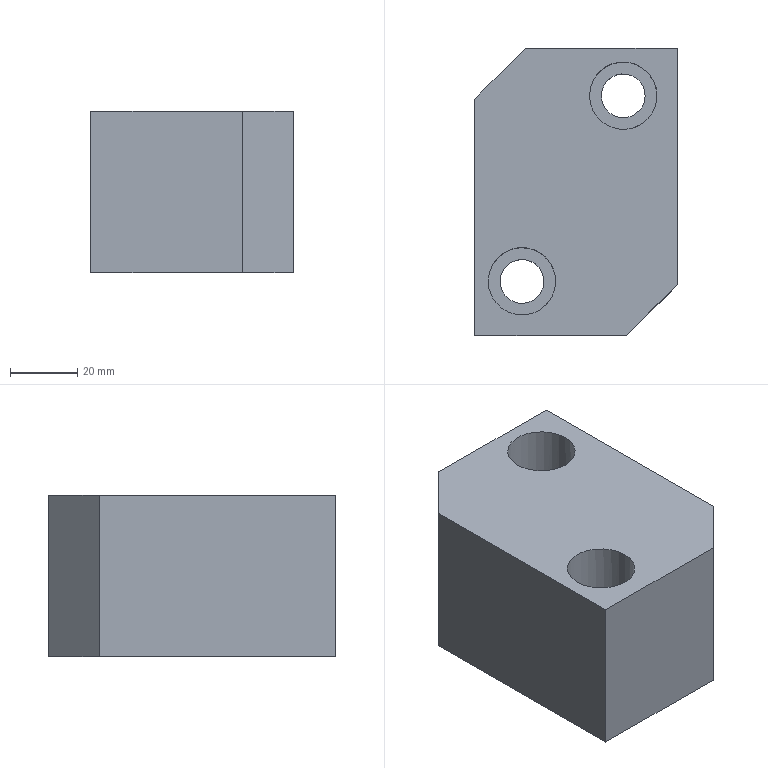Part | STEP file | gslz 2016.10.28-13_id778_x_t | 1 solid | 14 faces | box 60 x 85 x 48 mm | volume 211823 mm3 | plane 10 | cylinder 4 | commonest cylinder face diameters 13 x2 20 x2
STEP:
#1=CARTESIAN_POINT('',(0.,0.,0.));
#2=DIRECTION('',(0.,0.,1.));
#3=DIRECTION('',(1.,0.,0.));
#4=AXIS2_PLACEMENT_3D('',#1,#2,#3);
#5=CARTESIAN_POINT('',(-482.591,116.092,-48.));
#6=VERTEX_POINT('',#5);
#7=CARTESIAN_POINT('',(-481.5,122.5,-48.));
#8=DIRECTION('',(0.,0.,1.));
#9=DIRECTION('',(-0.1678,-0.9858,0.));
#10=AXIS2_PLACEMENT_3D('',#7,#8,#9);
#11=CIRCLE('',#10,6.5);
#12=CARTESIAN_POINT('',(-574.349,36.098,-48.));
#13=DIRECTION('',(0.,0.,1.));
#14=DIRECTION('',(1.,0.,0.));
#15=AXIS2_PLACEMENT_3D('',#12,#13,#14);
#16=PLANE('',#15);
#17=CARTESIAN_POINT('',(92.849,86.402));
#18=DIRECTION('',(-0.1678,-0.9858));
#19=AXIS2_PLACEMENT_2D('',#17,#18);
#20=CIRCLE('',#19,6.5);
#21=(GEOMETRIC_REPRESENTATION_CONTEXT(2)PARAMETRIC_REPRESENTATION_CONTEXT()REPRESENTATION_CONTEXT('',''));
#22=DEFINITIONAL_REPRESENTATION('',(#20),#21);
#23=PCURVE('',#16,#22);
#24=CARTESIAN_POINT('',(-481.5,122.5,-8.541));
#25=DIRECTION('',(0.,0.,-1.));
#26=DIRECTION('',(-1.,0.,0.));
#27=AXIS2_PLACEMENT_3D('',#24,#25,#26);
#28=CYLINDRICAL_SURFACE('',#27,6.5);
#29=CARTESIAN_POINT('',(11.164,39.459));
#30=DIRECTION('',(-1.,0.));
#31=VECTOR('',#30,1.);
#32=LINE('',#29,#31);
#33=(GEOMETRIC_REPRESENTATION_CONTEXT(2)PARAMETRIC_REPRESENTATION_CONTEXT()REPRESENTATION_CONTEXT('',''));
#34=DEFINITIONAL_REPRESENTATION('',(#32),#33);
#35=PCURVE('',#28,#34);
#36=SURFACE_CURVE('',#11,(#23,#35),.PCURVE_S1.);
#37=EDGE_CURVE('',#6,#6,#36,.T.);
#38=ORIENTED_EDGE('',*,*,#37,.T.);
#39=EDGE_LOOP('',(#38));
#40=FACE_BOUND('',#39,.T.);
#41=CARTESIAN_POINT('',(-452.591,171.092,-48.));
#42=VERTEX_POINT('',#41);
#43=CARTESIAN_POINT('',(-451.5,177.5,-48.));
#44=DIRECTION('',(0.,0.,1.));
#45=DIRECTION('',(-0.1678,-0.9858,0.));
#46=AXIS2_PLACEMENT_3D('',#43,#44,#45);
#47=CIRCLE('',#46,6.5);
#48=CARTESIAN_POINT('',(122.849,141.402));
#49=DIRECTION('',(-0.1678,-0.9858));
#50=AXIS2_PLACEMENT_2D('',#48,#49);
#51=CIRCLE('',#50,6.5);
#52=(GEOMETRIC_REPRESENTATION_CONTEXT(2)PARAMETRIC_REPRESENTATION_CONTEXT()REPRESENTATION_CONTEXT('',''));
#53=DEFINITIONAL_REPRESENTATION('',(#51),#52);
#54=PCURVE('',#16,#53);
#55=CARTESIAN_POINT('',(-451.5,177.5,-8.541));
#56=DIRECTION('',(0.,0.,-1.));
#57=DIRECTION('',(-1.,0.,0.));
#58=AXIS2_PLACEMENT_3D('',#55,#56,#57);
#59=CYLINDRICAL_SURFACE('',#58,6.5);
#60=CARTESIAN_POINT('',(11.164,39.459));
#61=DIRECTION('',(-1.,0.));
#62=VECTOR('',#61,1.);
#63=LINE('',#60,#62);
#64=(GEOMETRIC_REPRESENTATION_CONTEXT(2)PARAMETRIC_REPRESENTATION_CONTEXT()REPRESENTATION_CONTEXT('',''));
#65=DEFINITIONAL_REPRESENTATION('',(#63),#64);
#66=PCURVE('',#59,#65);
#67=SURFACE_CURVE('',#47,(#54,#66),.PCURVE_S1.);
#68=EDGE_CURVE('',#42,#42,#67,.T.);
#69=ORIENTED_EDGE('',*,*,#68,.T.);
#70=EDGE_LOOP('',(#69));
#71=FACE_BOUND('',#70,.T.);
#72=CARTESIAN_POINT('',(-495.5,176.5,-48.));
#73=VERTEX_POINT('',#72);
#74=CARTESIAN_POINT('',(-495.5,106.5,-48.));
#75=VERTEX_POINT('',#74);
#76=CARTESIAN_POINT('',(-495.5,151.5,-48.));
#77=DIRECTION('',(0.,-1.,0.));
#78=VECTOR('',#77,1.);
#79=LINE('',#76,#78);
#80=CARTESIAN_POINT('',(78.849,115.402));
#81=DIRECTION('',(0.,-1.));
#82=VECTOR('',#81,1.);
#83=LINE('',#80,#82);
#84=(GEOMETRIC_REPRESENTATION_CONTEXT(2)PARAMETRIC_REPRESENTATION_CONTEXT()REPRESENTATION_CONTEXT('',''));
#85=DEFINITIONAL_REPRESENTATION('',(#83),#84);
#86=PCURVE('',#16,#85);
#87=CARTESIAN_POINT('',(-495.5,151.5,-25.5));
#88=DIRECTION('',(1.,0.,0.));
#89=DIRECTION('',(0.,0.,-1.));
#90=AXIS2_PLACEMENT_3D('',#87,#88,#89);
#91=PLANE('',#90);
#92=CARTESIAN_POINT('',(22.5,0.));
#93=DIRECTION('',(0.,-1.));
#94=VECTOR('',#93,1.);
#95=LINE('',#92,#94);
#96=(GEOMETRIC_REPRESENTATION_CONTEXT(2)PARAMETRIC_REPRESENTATION_CONTEXT()REPRESENTATION_CONTEXT('',''));
#97=DEFINITIONAL_REPRESENTATION('',(#95),#96);
#98=PCURVE('',#91,#97);
#99=SURFACE_CURVE('',#79,(#86,#98),.PCURVE_S1.);
#100=EDGE_CURVE('',#73,#75,#99,.T.);
#101=ORIENTED_EDGE('',*,*,#100,.F.);
#102=CARTESIAN_POINT('',(-480.5,191.5,-48.));
#103=VERTEX_POINT('',#102);
#104=CARTESIAN_POINT('',(-495.5,176.5,-48.));
#105=DIRECTION('',(0.7071,0.7071,0.));
#106=VECTOR('',#105,1.);
#107=LINE('',#104,#106);
#108=CARTESIAN_POINT('',(78.849,140.402));
#109=DIRECTION('',(0.7071,0.7071));
#110=VECTOR('',#109,1.);
#111=LINE('',#108,#110);
#112=(GEOMETRIC_REPRESENTATION_CONTEXT(2)PARAMETRIC_REPRESENTATION_CONTEXT()REPRESENTATION_CONTEXT('',''));
#113=DEFINITIONAL_REPRESENTATION('',(#111),#112);
#114=PCURVE('',#16,#113);
#115=CARTESIAN_POINT('',(-495.5,176.5,-25.5));
#116=DIRECTION('',(-0.7071,0.7071,0.));
#117=DIRECTION('',(0.,0.,1.));
#118=AXIS2_PLACEMENT_3D('',#115,#116,#117);
#119=PLANE('',#118);
#120=CARTESIAN_POINT('',(-22.5,0.));
#121=DIRECTION('',(0.,1.));
#122=VECTOR('',#121,1.);
#123=LINE('',#120,#122);
#124=(GEOMETRIC_REPRESENTATION_CONTEXT(2)PARAMETRIC_REPRESENTATION_CONTEXT()REPRESENTATION_CONTEXT('',''));
#125=DEFINITIONAL_REPRESENTATION('',(#123),#124);
#126=PCURVE('',#119,#125);
#127=SURFACE_CURVE('',#107,(#114,#126),.PCURVE_S1.);
#128=EDGE_CURVE('',#73,#103,#127,.T.);
#129=ORIENTED_EDGE('',*,*,#128,.T.);
#130=CARTESIAN_POINT('',(-435.5,191.5,-48.));
#131=VERTEX_POINT('',#130);
#132=CARTESIAN_POINT('',(-574.349,191.5,-48.));
#133=DIRECTION('',(-1.,0.,0.));
#134=VECTOR('',#133,1.);
#135=LINE('',#132,#134);
#136=CARTESIAN_POINT('',(0.,155.402));
#137=DIRECTION('',(-1.,0.));
#138=VECTOR('',#137,1.);
#139=LINE('',#136,#138);
#140=(GEOMETRIC_REPRESENTATION_CONTEXT(2)PARAMETRIC_REPRESENTATION_CONTEXT()REPRESENTATION_CONTEXT('',''));
#141=DEFINITIONAL_REPRESENTATION('',(#139),#140);
#142=PCURVE('',#16,#141);
#143=CARTESIAN_POINT('',(-441.5,191.5,-43.));
#144=DIRECTION('',(0.,1.,0.));
#145=DIRECTION('',(-1.,0.,0.));
#146=AXIS2_PLACEMENT_3D('',#143,#144,#145);
#147=PLANE('',#146);
#148=CARTESIAN_POINT('',(132.849,-5.));
#149=DIRECTION('',(1.,0.));
#150=VECTOR('',#149,1.);
#151=LINE('',#148,#150);
#152=(GEOMETRIC_REPRESENTATION_CONTEXT(2)PARAMETRIC_REPRESENTATION_CONTEXT()REPRESENTATION_CONTEXT('',''));
#153=DEFINITIONAL_REPRESENTATION('',(#151),#152);
#154=PCURVE('',#147,#153);
#155=SURFACE_CURVE('',#135,(#142,#154),.PCURVE_S1.);
#156=EDGE_CURVE('',#131,#103,#155,.T.);
#157=ORIENTED_EDGE('',*,*,#156,.F.);
#158=CARTESIAN_POINT('',(-435.5,121.5,-48.));
#159=VERTEX_POINT('',#158);
#160=CARTESIAN_POINT('',(-435.5,36.098,-48.));
#161=DIRECTION('',(0.,1.,0.));
#162=VECTOR('',#161,1.);
#163=LINE('',#160,#162);
#164=CARTESIAN_POINT('',(138.849,0.));
#165=DIRECTION('',(0.,1.));
#166=VECTOR('',#165,1.);
#167=LINE('',#164,#166);
#168=(GEOMETRIC_REPRESENTATION_CONTEXT(2)PARAMETRIC_REPRESENTATION_CONTEXT()REPRESENTATION_CONTEXT('',''));
#169=DEFINITIONAL_REPRESENTATION('',(#167),#168);
#170=PCURVE('',#16,#169);
#171=CARTESIAN_POINT('',(-435.5,106.5,-43.));
#172=DIRECTION('',(1.,0.,0.));
#173=DIRECTION('',(0.,1.,0.));
#174=AXIS2_PLACEMENT_3D('',#171,#172,#173);
#175=PLANE('',#174);
#176=CARTESIAN_POINT('',(-70.402,-5.));
#177=DIRECTION('',(1.,0.));
#178=VECTOR('',#177,1.);
#179=LINE('',#176,#178);
#180=(GEOMETRIC_REPRESENTATION_CONTEXT(2)PARAMETRIC_REPRESENTATION_CONTEXT()REPRESENTATION_CONTEXT('',''));
#181=DEFINITIONAL_REPRESENTATION('',(#179),#180);
#182=PCURVE('',#175,#181);
#183=SURFACE_CURVE('',#163,(#170,#182),.PCURVE_S1.);
#184=EDGE_CURVE('',#159,#131,#183,.T.);
#185=ORIENTED_EDGE('',*,*,#184,.F.);
#186=CARTESIAN_POINT('',(-450.5,106.5,-48.));
#187=VERTEX_POINT('',#186);
#188=CARTESIAN_POINT('',(-450.5,106.5,-48.));
#189=DIRECTION('',(-0.7071,-0.7071,0.));
#190=VECTOR('',#189,1.);
#191=LINE('',#188,#190);
#192=CARTESIAN_POINT('',(123.849,70.402));
#193=DIRECTION('',(-0.7071,-0.7071));
#194=VECTOR('',#193,1.);
#195=LINE('',#192,#194);
#196=(GEOMETRIC_REPRESENTATION_CONTEXT(2)PARAMETRIC_REPRESENTATION_CONTEXT()REPRESENTATION_CONTEXT('',''));
#197=DEFINITIONAL_REPRESENTATION('',(#195),#196);
#198=PCURVE('',#16,#197);
#199=CARTESIAN_POINT('',(-450.5,106.5,-43.));
#200=DIRECTION('',(-0.7071,0.7071,0.));
#201=DIRECTION('',(0.,0.,1.));
#202=AXIS2_PLACEMENT_3D('',#199,#200,#201);
#203=PLANE('',#202);
#204=CARTESIAN_POINT('',(-5.,0.));
#205=DIRECTION('',(0.,-1.));
#206=VECTOR('',#205,1.);
#207=LINE('',#204,#206);
#208=(GEOMETRIC_REPRESENTATION_CONTEXT(2)PARAMETRIC_REPRESENTATION_CONTEXT()REPRESENTATION_CONTEXT('',''));
#209=DEFINITIONAL_REPRESENTATION('',(#207),#208);
#210=PCURVE('',#203,#209);
#211=SURFACE_CURVE('',#191,(#198,#210),.PCURVE_S1.);
#212=EDGE_CURVE('',#159,#187,#211,.T.);
#213=ORIENTED_EDGE('',*,*,#212,.T.);
#214=CARTESIAN_POINT('',(-574.349,106.5,-48.));
#215=DIRECTION('',(1.,0.,0.));
#216=VECTOR('',#215,1.);
#217=LINE('',#214,#216);
#218=CARTESIAN_POINT('',(0.,70.402));
#219=DIRECTION('',(1.,0.));
#220=VECTOR('',#219,1.);
#221=LINE('',#218,#220);
#222=(GEOMETRIC_REPRESENTATION_CONTEXT(2)PARAMETRIC_REPRESENTATION_CONTEXT()REPRESENTATION_CONTEXT('',''));
#223=DEFINITIONAL_REPRESENTATION('',(#221),#222);
#224=PCURVE('',#16,#223);
#225=CARTESIAN_POINT('',(-631.5,106.5,-43.));
#226=DIRECTION('',(0.,-1.,0.));
#227=DIRECTION('',(0.,0.,1.));
#228=AXIS2_PLACEMENT_3D('',#225,#226,#227);
#229=PLANE('',#228);
#230=CARTESIAN_POINT('',(-5.,-57.151));
#231=DIRECTION('',(0.,-1.));
#232=VECTOR('',#231,1.);
#233=LINE('',#230,#232);
#234=(GEOMETRIC_REPRESENTATION_CONTEXT(2)PARAMETRIC_REPRESENTATION_CONTEXT()REPRESENTATION_CONTEXT('',''));
#235=DEFINITIONAL_REPRESENTATION('',(#233),#234);
#236=PCURVE('',#229,#235);
#237=SURFACE_CURVE('',#217,(#224,#236),.PCURVE_S1.);
#238=EDGE_CURVE('',#75,#187,#237,.T.);
#239=ORIENTED_EDGE('',*,*,#238,.F.);
#240=EDGE_LOOP('',(#101,#129,#157,#185,#213,#239));
#241=FACE_BOUND('',#240,.T.);
#242=ADVANCED_FACE('',(#40,#71,#241),#16,.F.);
#243=ORIENTED_EDGE('',*,*,#156,.T.);
#244=CARTESIAN_POINT('',(-480.5,191.5,0.));
#245=VERTEX_POINT('',#244);
#246=CARTESIAN_POINT('',(-480.5,191.5,0.));
#247=DIRECTION('',(0.,0.,1.));
#248=VECTOR('',#247,1.);
#249=LINE('',#246,#248);
#250=CARTESIAN_POINT('',(39.,43.));
#251=DIRECTION('',(0.,1.));
#252=VECTOR('',#251,1.);
#253=LINE('',#250,#252);
#254=(GEOMETRIC_REPRESENTATION_CONTEXT(2)PARAMETRIC_REPRESENTATION_CONTEXT()REPRESENTATION_CONTEXT('',''));
#255=DEFINITIONAL_REPRESENTATION('',(#253),#254);
#256=PCURVE('',#147,#255);
#257=CARTESIAN_POINT('',(25.5,21.213));
#258=DIRECTION('',(1.,0.));
#259=VECTOR('',#258,1.);
#260=LINE('',#257,#259);
#261=(GEOMETRIC_REPRESENTATION_CONTEXT(2)PARAMETRIC_REPRESENTATION_CONTEXT()REPRESENTATION_CONTEXT('',''));
#262=DEFINITIONAL_REPRESENTATION('',(#260),#261);
#263=PCURVE('',#119,#262);
#264=SURFACE_CURVE('',#249,(#256,#263),.PCURVE_S1.);
#265=EDGE_CURVE('',#103,#245,#264,.T.);
#266=ORIENTED_EDGE('',*,*,#265,.T.);
#267=CARTESIAN_POINT('',(-435.5,191.5,0.));
#268=VERTEX_POINT('',#267);
#269=CARTESIAN_POINT('',(-441.5,191.5,0.));
#270=DIRECTION('',(-1.,0.,0.));
#271=VECTOR('',#270,1.);
#272=LINE('',#269,#271);
#273=CARTESIAN_POINT('',(0.,43.));
#274=DIRECTION('',(1.,0.));
#275=VECTOR('',#274,1.);
#276=LINE('',#273,#275);
#277=(GEOMETRIC_REPRESENTATION_CONTEXT(2)PARAMETRIC_REPRESENTATION_CONTEXT()REPRESENTATION_CONTEXT('',''));
#278=DEFINITIONAL_REPRESENTATION('',(#276),#277);
#279=PCURVE('',#147,#278);
#280=CARTESIAN_POINT('',(-540.228,222.5,0.));
#281=DIRECTION('',(0.,0.,1.));
#282=DIRECTION('',(0.,1.,0.));
#283=AXIS2_PLACEMENT_3D('',#280,#281,#282);
#284=PLANE('',#283);
#285=CARTESIAN_POINT('',(-31.,-98.728));
#286=DIRECTION('',(0.,1.));
#287=VECTOR('',#286,1.);
#288=LINE('',#285,#287);
#289=(GEOMETRIC_REPRESENTATION_CONTEXT(2)PARAMETRIC_REPRESENTATION_CONTEXT()REPRESENTATION_CONTEXT('',''));
#290=DEFINITIONAL_REPRESENTATION('',(#288),#289);
#291=PCURVE('',#284,#290);
#292=SURFACE_CURVE('',#272,(#279,#291),.PCURVE_S1.);
#293=EDGE_CURVE('',#268,#245,#292,.T.);
#294=ORIENTED_EDGE('',*,*,#293,.F.);
#295=CARTESIAN_POINT('',(-435.5,191.5,-43.));
#296=DIRECTION('',(0.,0.,1.));
#297=VECTOR('',#296,1.);
#298=LINE('',#295,#297);
#299=CARTESIAN_POINT('',(-6.,0.));
#300=DIRECTION('',(0.,1.));
#301=VECTOR('',#300,1.);
#302=LINE('',#299,#301);
#303=(GEOMETRIC_REPRESENTATION_CONTEXT(2)PARAMETRIC_REPRESENTATION_CONTEXT()REPRESENTATION_CONTEXT('',''));
#304=DEFINITIONAL_REPRESENTATION('',(#302),#303);
#305=PCURVE('',#147,#304);
#306=CARTESIAN_POINT('',(85.,0.));
#307=DIRECTION('',(0.,1.));
#308=VECTOR('',#307,1.);
#309=LINE('',#306,#308);
#310=(GEOMETRIC_REPRESENTATION_CONTEXT(2)PARAMETRIC_REPRESENTATION_CONTEXT()REPRESENTATION_CONTEXT('',''));
#311=DEFINITIONAL_REPRESENTATION('',(#309),#310);
#312=PCURVE('',#175,#311);
#313=SURFACE_CURVE('',#298,(#305,#312),.PCURVE_S1.);
#314=EDGE_CURVE('',#131,#268,#313,.T.);
#315=ORIENTED_EDGE('',*,*,#314,.F.);
#316=EDGE_LOOP('',(#243,#266,#294,#315));
#317=FACE_BOUND('',#316,.T.);
#318=ADVANCED_FACE('',(#317),#147,.T.);
#319=CARTESIAN_POINT('',(-435.5,121.5,0.));
#320=VERTEX_POINT('',#319);
#321=CARTESIAN_POINT('',(-435.5,106.5,0.));
#322=DIRECTION('',(0.,1.,0.));
#323=VECTOR('',#322,1.);
#324=LINE('',#321,#323);
#325=CARTESIAN_POINT('',(0.,43.));
#326=DIRECTION('',(1.,0.));
#327=VECTOR('',#326,1.);
#328=LINE('',#325,#327);
#329=(GEOMETRIC_REPRESENTATION_CONTEXT(2)PARAMETRIC_REPRESENTATION_CONTEXT()REPRESENTATION_CONTEXT('',''));
#330=DEFINITIONAL_REPRESENTATION('',(#328),#329);
#331=PCURVE('',#175,#330);
#332=CARTESIAN_POINT('',(-116.,-104.728));
#333=DIRECTION('',(1.,0.));
#334=VECTOR('',#333,1.);
#335=LINE('',#332,#334);
#336=(GEOMETRIC_REPRESENTATION_CONTEXT(2)PARAMETRIC_REPRESENTATION_CONTEXT()REPRESENTATION_CONTEXT('',''));
#337=DEFINITIONAL_REPRESENTATION('',(#335),#336);
#338=PCURVE('',#284,#337);
#339=SURFACE_CURVE('',#324,(#331,#338),.PCURVE_S1.);
#340=EDGE_CURVE('',#320,#268,#339,.T.);
#341=ORIENTED_EDGE('',*,*,#340,.F.);
#342=CARTESIAN_POINT('',(-435.5,121.5,-43.));
#343=DIRECTION('',(0.,0.,-1.));
#344=VECTOR('',#343,1.);
#345=LINE('',#342,#344);
#346=CARTESIAN_POINT('',(15.,0.));
#347=DIRECTION('',(0.,-1.));
#348=VECTOR('',#347,1.);
#349=LINE('',#346,#348);
#350=(GEOMETRIC_REPRESENTATION_CONTEXT(2)PARAMETRIC_REPRESENTATION_CONTEXT()REPRESENTATION_CONTEXT('',''));
#351=DEFINITIONAL_REPRESENTATION('',(#349),#350);
#352=PCURVE('',#175,#351);
#353=CARTESIAN_POINT('',(0.,21.213));
#354=DIRECTION('',(-1.,0.));
#355=VECTOR('',#354,1.);
#356=LINE('',#353,#355);
#357=(GEOMETRIC_REPRESENTATION_CONTEXT(2)PARAMETRIC_REPRESENTATION_CONTEXT()REPRESENTATION_CONTEXT('',''));
#358=DEFINITIONAL_REPRESENTATION('',(#356),#357);
#359=PCURVE('',#203,#358);
#360=SURFACE_CURVE('',#345,(#352,#359),.PCURVE_S1.);
#361=EDGE_CURVE('',#320,#159,#360,.T.);
#362=ORIENTED_EDGE('',*,*,#361,.T.);
#363=ORIENTED_EDGE('',*,*,#184,.T.);
#364=ORIENTED_EDGE('',*,*,#314,.T.);
#365=EDGE_LOOP('',(#341,#362,#363,#364));
#366=FACE_BOUND('',#365,.T.);
#367=ADVANCED_FACE('',(#366),#175,.T.);
#368=ORIENTED_EDGE('',*,*,#238,.T.);
#369=CARTESIAN_POINT('',(-450.5,106.5,0.));
#370=VERTEX_POINT('',#369);
#371=CARTESIAN_POINT('',(-450.5,106.5,-43.));
#372=DIRECTION('',(0.,0.,1.));
#373=VECTOR('',#372,1.);
#374=LINE('',#371,#373);
#375=CARTESIAN_POINT('',(0.,-181.));
#376=DIRECTION('',(1.,0.));
#377=VECTOR('',#376,1.);
#378=LINE('',#375,#377);
#379=(GEOMETRIC_REPRESENTATION_CONTEXT(2)PARAMETRIC_REPRESENTATION_CONTEXT()REPRESENTATION_CONTEXT('',''));
#380=DEFINITIONAL_REPRESENTATION('',(#378),#379);
#381=PCURVE('',#229,#380);
#382=CARTESIAN_POINT('',(0.,0.));
#383=DIRECTION('',(1.,0.));
#384=VECTOR('',#383,1.);
#385=LINE('',#382,#384);
#386=(GEOMETRIC_REPRESENTATION_CONTEXT(2)PARAMETRIC_REPRESENTATION_CONTEXT()REPRESENTATION_CONTEXT('',''));
#387=DEFINITIONAL_REPRESENTATION('',(#385),#386);
#388=PCURVE('',#203,#387);
#389=SURFACE_CURVE('',#374,(#381,#388),.PCURVE_S1.);
#390=EDGE_CURVE('',#187,#370,#389,.T.);
#391=ORIENTED_EDGE('',*,*,#390,.T.);
#392=CARTESIAN_POINT('',(-495.5,106.5,0.));
#393=VERTEX_POINT('',#392);
#394=CARTESIAN_POINT('',(-631.5,106.5,0.));
#395=DIRECTION('',(1.,0.,0.));
#396=VECTOR('',#395,1.);
#397=LINE('',#394,#396);
#398=CARTESIAN_POINT('',(43.,0.));
#399=DIRECTION('',(0.,-1.));
#400=VECTOR('',#399,1.);
#401=LINE('',#398,#400);
#402=(GEOMETRIC_REPRESENTATION_CONTEXT(2)PARAMETRIC_REPRESENTATION_CONTEXT()REPRESENTATION_CONTEXT('',''));
#403=DEFINITIONAL_REPRESENTATION('',(#401),#402);
#404=PCURVE('',#229,#403);
#405=CARTESIAN_POINT('',(-116.,91.272));
#406=DIRECTION('',(0.,-1.));
#407=VECTOR('',#406,1.);
#408=LINE('',#405,#407);
#409=(GEOMETRIC_REPRESENTATION_CONTEXT(2)PARAMETRIC_REPRESENTATION_CONTEXT()REPRESENTATION_CONTEXT('',''));
#410=DEFINITIONAL_REPRESENTATION('',(#408),#409);
#411=PCURVE('',#284,#410);
#412=SURFACE_CURVE('',#397,(#404,#411),.PCURVE_S1.);
#413=EDGE_CURVE('',#393,#370,#412,.T.);
#414=ORIENTED_EDGE('',*,*,#413,.F.);
#415=CARTESIAN_POINT('',(-495.5,106.5,-43.));
#416=DIRECTION('',(0.,0.,-1.));
#417=VECTOR('',#416,1.);
#418=LINE('',#415,#417);
#419=CARTESIAN_POINT('',(0.,-136.));
#420=DIRECTION('',(-1.,0.));
#421=VECTOR('',#420,1.);
#422=LINE('',#419,#421);
#423=(GEOMETRIC_REPRESENTATION_CONTEXT(2)PARAMETRIC_REPRESENTATION_CONTEXT()REPRESENTATION_CONTEXT('',''));
#424=DEFINITIONAL_REPRESENTATION('',(#422),#423);
#425=PCURVE('',#229,#424);
#426=CARTESIAN_POINT('',(17.5,-45.));
#427=DIRECTION('',(1.,0.));
#428=VECTOR('',#427,1.);
#429=LINE('',#426,#428);
#430=(GEOMETRIC_REPRESENTATION_CONTEXT(2)PARAMETRIC_REPRESENTATION_CONTEXT()REPRESENTATION_CONTEXT('',''));
#431=DEFINITIONAL_REPRESENTATION('',(#429),#430);
#432=PCURVE('',#91,#431);
#433=SURFACE_CURVE('',#418,(#425,#432),.PCURVE_S1.);
#434=EDGE_CURVE('',#393,#75,#433,.T.);
#435=ORIENTED_EDGE('',*,*,#434,.T.);
#436=EDGE_LOOP('',(#368,#391,#414,#435));
#437=FACE_BOUND('',#436,.T.);
#438=ADVANCED_FACE('',(#437),#229,.T.);
#439=CARTESIAN_POINT('',(-495.5,176.5,0.));
#440=VERTEX_POINT('',#439);
#441=CARTESIAN_POINT('',(-495.5,222.5,0.));
#442=DIRECTION('',(0.,1.,0.));
#443=VECTOR('',#442,1.);
#444=LINE('',#441,#443);
#445=CARTESIAN_POINT('',(-25.5,71.));
#446=DIRECTION('',(0.,1.));
#447=VECTOR('',#446,1.);
#448=LINE('',#445,#447);
#449=(GEOMETRIC_REPRESENTATION_CONTEXT(2)PARAMETRIC_REPRESENTATION_CONTEXT()REPRESENTATION_CONTEXT('',''));
#450=DEFINITIONAL_REPRESENTATION('',(#448),#449);
#451=PCURVE('',#91,#450);
#452=CARTESIAN_POINT('',(0.,-44.728));
#453=DIRECTION('',(1.,0.));
#454=VECTOR('',#453,1.);
#455=LINE('',#452,#454);
#456=(GEOMETRIC_REPRESENTATION_CONTEXT(2)PARAMETRIC_REPRESENTATION_CONTEXT()REPRESENTATION_CONTEXT('',''));
#457=DEFINITIONAL_REPRESENTATION('',(#455),#456);
#458=PCURVE('',#284,#457);
#459=SURFACE_CURVE('',#444,(#451,#458),.PCURVE_S1.);
#460=EDGE_CURVE('',#393,#440,#459,.T.);
#461=ORIENTED_EDGE('',*,*,#460,.T.);
#462=CARTESIAN_POINT('',(-495.5,176.5,-48.));
#463=DIRECTION('',(0.,0.,-1.));
#464=VECTOR('',#463,1.);
#465=LINE('',#462,#464);
#466=CARTESIAN_POINT('',(22.5,25.));
#467=DIRECTION('',(1.,0.));
#468=VECTOR('',#467,1.);
#469=LINE('',#466,#468);
#470=(GEOMETRIC_REPRESENTATION_CONTEXT(2)PARAMETRIC_REPRESENTATION_CONTEXT()REPRESENTATION_CONTEXT('',''));
#471=DEFINITIONAL_REPRESENTATION('',(#469),#470);
#472=PCURVE('',#91,#471);
#473=CARTESIAN_POINT('',(-22.5,0.));
#474=DIRECTION('',(-1.,0.));
#475=VECTOR('',#474,1.);
#476=LINE('',#473,#475);
#477=(GEOMETRIC_REPRESENTATION_CONTEXT(2)PARAMETRIC_REPRESENTATION_CONTEXT()REPRESENTATION_CONTEXT('',''));
#478=DEFINITIONAL_REPRESENTATION('',(#476),#477);
#479=PCURVE('',#119,#478);
#480=SURFACE_CURVE('',#465,(#472,#479),.PCURVE_S1.);
#481=EDGE_CURVE('',#440,#73,#480,.T.);
#482=ORIENTED_EDGE('',*,*,#481,.T.);
#483=ORIENTED_EDGE('',*,*,#100,.T.);
#484=ORIENTED_EDGE('',*,*,#434,.F.);
#485=EDGE_LOOP('',(#461,#482,#483,#484));
#486=FACE_BOUND('',#485,.T.);
#487=ADVANCED_FACE('',(#486),#91,.F.);
#488=CARTESIAN_POINT('',(-471.5,122.5,0.));
#489=VERTEX_POINT('',#488);
#490=CARTESIAN_POINT('',(-483.178,112.642,0.));
#491=VERTEX_POINT('',#490);
#492=CARTESIAN_POINT('',(-481.5,122.5,0.));
#493=DIRECTION('',(0.,0.,1.));
#494=DIRECTION('',(1.,0.,0.));
#495=AXIS2_PLACEMENT_3D('',#492,#493,#494);
#496=CIRCLE('',#495,10.);
#497=CARTESIAN_POINT('',(-100.,-58.728));
#498=DIRECTION('',(0.,-1.));
#499=AXIS2_PLACEMENT_2D('',#497,#498);
#500=CIRCLE('',#499,10.);
#501=(GEOMETRIC_REPRESENTATION_CONTEXT(2)PARAMETRIC_REPRESENTATION_CONTEXT()REPRESENTATION_CONTEXT('',''));
#502=DEFINITIONAL_REPRESENTATION('',(#500),#501);
#503=PCURVE('',#284,#502);
#504=CARTESIAN_POINT('',(-481.5,122.5,-8.541));
#505=DIRECTION('',(0.,0.,-1.));
#506=DIRECTION('',(-1.,0.,0.));
#507=AXIS2_PLACEMENT_3D('',#504,#505,#506);
#508=CYLINDRICAL_SURFACE('',#507,10.);
#509=CARTESIAN_POINT('',(9.425,-8.541));
#510=DIRECTION('',(-1.,0.));
#511=VECTOR('',#510,1.);
#512=LINE('',#509,#511);
#513=(GEOMETRIC_REPRESENTATION_CONTEXT(2)PARAMETRIC_REPRESENTATION_CONTEXT()REPRESENTATION_CONTEXT('',''));
#514=DEFINITIONAL_REPRESENTATION('',(#512),#513);
#515=PCURVE('',#508,#514);
#516=SURFACE_CURVE('',#496,(#503,#515),.PCURVE_S1.);
#517=EDGE_CURVE('',#489,#491,#516,.T.);
#518=ORIENTED_EDGE('',*,*,#517,.F.);
#519=CARTESIAN_POINT('',(-481.5,122.5,0.));
#520=DIRECTION('',(0.,0.,1.));
#521=DIRECTION('',(1.,0.,0.));
#522=AXIS2_PLACEMENT_3D('',#519,#520,#521);
#523=CIRCLE('',#522,10.);
#524=CARTESIAN_POINT('',(-100.,-58.728));
#525=DIRECTION('',(0.,-1.));
#526=AXIS2_PLACEMENT_2D('',#524,#525);
#527=CIRCLE('',#526,10.);
#528=(GEOMETRIC_REPRESENTATION_CONTEXT(2)PARAMETRIC_REPRESENTATION_CONTEXT()REPRESENTATION_CONTEXT('',''));
#529=DEFINITIONAL_REPRESENTATION('',(#527),#528);
#530=PCURVE('',#284,#529);
#531=CARTESIAN_POINT('',(15.708,-8.541));
#532=DIRECTION('',(-1.,0.));
#533=VECTOR('',#532,1.);
#534=LINE('',#531,#533);
#535=(GEOMETRIC_REPRESENTATION_CONTEXT(2)PARAMETRIC_REPRESENTATION_CONTEXT()REPRESENTATION_CONTEXT('',''));
#536=DEFINITIONAL_REPRESENTATION('',(#534),#535);
#537=PCURVE('',#508,#536);
#538=SURFACE_CURVE('',#523,(#530,#537),.PCURVE_S1.);
#539=EDGE_CURVE('',#491,#489,#538,.T.);
#540=ORIENTED_EDGE('',*,*,#539,.F.);
#541=EDGE_LOOP('',(#518,#540));
#542=FACE_BOUND('',#541,.T.);
#543=CARTESIAN_POINT('',(-441.5,177.5,0.));
#544=VERTEX_POINT('',#543);
#545=CARTESIAN_POINT('',(-453.178,167.642,0.));
#546=VERTEX_POINT('',#545);
#547=CARTESIAN_POINT('',(-451.5,177.5,0.));
#548=DIRECTION('',(0.,0.,1.));
#549=DIRECTION('',(1.,0.,0.));
#550=AXIS2_PLACEMENT_3D('',#547,#548,#549);
#551=CIRCLE('',#550,10.);
#552=CARTESIAN_POINT('',(-45.,-88.728));
#553=DIRECTION('',(0.,-1.));
#554=AXIS2_PLACEMENT_2D('',#552,#553);
#555=CIRCLE('',#554,10.);
#556=(GEOMETRIC_REPRESENTATION_CONTEXT(2)PARAMETRIC_REPRESENTATION_CONTEXT()REPRESENTATION_CONTEXT('',''));
#557=DEFINITIONAL_REPRESENTATION('',(#555),#556);
#558=PCURVE('',#284,#557);
#559=CARTESIAN_POINT('',(-451.5,177.5,-8.541));
#560=DIRECTION('',(0.,0.,-1.));
#561=DIRECTION('',(-1.,0.,0.));
#562=AXIS2_PLACEMENT_3D('',#559,#560,#561);
#563=CYLINDRICAL_SURFACE('',#562,10.);
#564=CARTESIAN_POINT('',(9.425,-8.541));
#565=DIRECTION('',(-1.,0.));
#566=VECTOR('',#565,1.);
#567=LINE('',#564,#566);
#568=(GEOMETRIC_REPRESENTATION_CONTEXT(2)PARAMETRIC_REPRESENTATION_CONTEXT()REPRESENTATION_CONTEXT('',''));
#569=DEFINITIONAL_REPRESENTATION('',(#567),#568);
#570=PCURVE('',#563,#569);
#571=SURFACE_CURVE('',#551,(#558,#570),.PCURVE_S1.);
#572=EDGE_CURVE('',#544,#546,#571,.T.);
#573=ORIENTED_EDGE('',*,*,#572,.F.);
#574=CARTESIAN_POINT('',(-451.5,177.5,0.));
#575=DIRECTION('',(0.,0.,1.));
#576=DIRECTION('',(1.,0.,0.));
#577=AXIS2_PLACEMENT_3D('',#574,#575,#576);
#578=CIRCLE('',#577,10.);
#579=CARTESIAN_POINT('',(-45.,-88.728));
#580=DIRECTION('',(0.,-1.));
#581=AXIS2_PLACEMENT_2D('',#579,#580);
#582=CIRCLE('',#581,10.);
#583=(GEOMETRIC_REPRESENTATION_CONTEXT(2)PARAMETRIC_REPRESENTATION_CONTEXT()REPRESENTATION_CONTEXT('',''));
#584=DEFINITIONAL_REPRESENTATION('',(#582),#583);
#585=PCURVE('',#284,#584);
#586=CARTESIAN_POINT('',(15.708,-8.541));
#587=DIRECTION('',(-1.,0.));
#588=VECTOR('',#587,1.);
#589=LINE('',#586,#588);
#590=(GEOMETRIC_REPRESENTATION_CONTEXT(2)PARAMETRIC_REPRESENTATION_CONTEXT()REPRESENTATION_CONTEXT('',''));
#591=DEFINITIONAL_REPRESENTATION('',(#589),#590);
#592=PCURVE('',#563,#591);
#593=SURFACE_CURVE('',#578,(#585,#592),.PCURVE_S1.);
#594=EDGE_CURVE('',#546,#544,#593,.T.);
#595=ORIENTED_EDGE('',*,*,#594,.F.);
#596=EDGE_LOOP('',(#573,#595));
#597=FACE_BOUND('',#596,.T.);
#598=ORIENTED_EDGE('',*,*,#293,.T.);
#599=CARTESIAN_POINT('',(-494.864,177.136,0.));
#600=DIRECTION('',(-0.7071,-0.7071,0.));
#601=VECTOR('',#600,1.);
#602=LINE('',#599,#601);
#603=CARTESIAN_POINT('',(-45.364,-45.364));
#604=DIRECTION('',(-0.7071,0.7071));
#605=VECTOR('',#604,1.);
#606=LINE('',#603,#605);
#607=(GEOMETRIC_REPRESENTATION_CONTEXT(2)PARAMETRIC_REPRESENTATION_CONTEXT()REPRESENTATION_CONTEXT('',''));
#608=DEFINITIONAL_REPRESENTATION('',(#606),#607);
#609=PCURVE('',#284,#608);
#610=CARTESIAN_POINT('',(25.5,0.8995));
#611=DIRECTION('',(0.,-1.));
#612=VECTOR('',#611,1.);
#613=LINE('',#610,#612);
#614=(GEOMETRIC_REPRESENTATION_CONTEXT(2)PARAMETRIC_REPRESENTATION_CONTEXT()REPRESENTATION_CONTEXT('',''));
#615=DEFINITIONAL_REPRESENTATION('',(#613),#614);
#616=PCURVE('',#119,#615);
#617=SURFACE_CURVE('',#602,(#609,#616),.PCURVE_S1.);
#618=EDGE_CURVE('',#245,#440,#617,.T.);
#619=ORIENTED_EDGE('',*,*,#618,.T.);
#620=ORIENTED_EDGE('',*,*,#460,.F.);
#621=ORIENTED_EDGE('',*,*,#413,.T.);
#622=CARTESIAN_POINT('',(-437.364,119.636,0.));
#623=DIRECTION('',(0.7071,0.7071,0.));
#624=VECTOR('',#623,1.);
#625=LINE('',#622,#624);
#626=CARTESIAN_POINT('',(-102.864,-102.864));
#627=DIRECTION('',(0.7071,-0.7071));
#628=VECTOR('',#627,1.);
#629=LINE('',#626,#628);
#630=(GEOMETRIC_REPRESENTATION_CONTEXT(2)PARAMETRIC_REPRESENTATION_CONTEXT()REPRESENTATION_CONTEXT('',''));
#631=DEFINITIONAL_REPRESENTATION('',(#629),#630);
#632=PCURVE('',#284,#631);
#633=CARTESIAN_POINT('',(43.,18.577));
#634=DIRECTION('',(0.,1.));
#635=VECTOR('',#634,1.);
#636=LINE('',#633,#635);
#637=(GEOMETRIC_REPRESENTATION_CONTEXT(2)PARAMETRIC_REPRESENTATION_CONTEXT()REPRESENTATION_CONTEXT('',''));
#638=DEFINITIONAL_REPRESENTATION('',(#636),#637);
#639=PCURVE('',#203,#638);
#640=SURFACE_CURVE('',#625,(#632,#639),.PCURVE_S1.);
#641=EDGE_CURVE('',#370,#320,#640,.T.);
#642=ORIENTED_EDGE('',*,*,#641,.T.);
#643=ORIENTED_EDGE('',*,*,#340,.T.);
#644=EDGE_LOOP('',(#598,#619,#620,#621,#642,#643));
#645=FACE_BOUND('',#644,.T.);
#646=ADVANCED_FACE('',(#542,#597,#645),#284,.T.);
#647=CARTESIAN_POINT('',(-452.591,171.092,-26.));
#648=VERTEX_POINT('',#647);
#649=CARTESIAN_POINT('',(-451.5,177.5,-26.));
#650=DIRECTION('',(0.,0.,1.));
#651=DIRECTION('',(-0.1678,-0.9858,0.));
#652=AXIS2_PLACEMENT_3D('',#649,#650,#651);
#653=CIRCLE('',#652,6.5);
#654=CARTESIAN_POINT('',(-451.5,177.5,-26.));
#655=DIRECTION('',(0.,0.,1.));
#656=DIRECTION('',(-0.1678,-0.9858,0.));
#657=AXIS2_PLACEMENT_3D('',#654,#655,#656);
#658=PLANE('',#657);
#659=CARTESIAN_POINT('',(0.,0.));
#660=DIRECTION('',(1.,0.));
#661=AXIS2_PLACEMENT_2D('',#659,#660);
#662=CIRCLE('',#661,6.5);
#663=(GEOMETRIC_REPRESENTATION_CONTEXT(2)PARAMETRIC_REPRESENTATION_CONTEXT()REPRESENTATION_CONTEXT('',''));
#664=DEFINITIONAL_REPRESENTATION('',(#662),#663);
#665=PCURVE('',#658,#664);
#666=CARTESIAN_POINT('',(11.164,17.459));
#667=DIRECTION('',(-1.,0.));
#668=VECTOR('',#667,1.);
#669=LINE('',#666,#668);
#670=(GEOMETRIC_REPRESENTATION_CONTEXT(2)PARAMETRIC_REPRESENTATION_CONTEXT()REPRESENTATION_CONTEXT('',''));
#671=DEFINITIONAL_REPRESENTATION('',(#669),#670);
#672=PCURVE('',#59,#671);
#673=SURFACE_CURVE('',#653,(#665,#672),.PCURVE_S1.);
#674=EDGE_CURVE('',#648,#648,#673,.T.);
#675=ORIENTED_EDGE('',*,*,#674,.F.);
#676=EDGE_LOOP('',(#675));
#677=FACE_BOUND('',#676,.T.);
#678=CARTESIAN_POINT('',(-453.178,167.642,-26.));
#679=VERTEX_POINT('',#678);
#680=CARTESIAN_POINT('',(-451.5,177.5,-26.));
#681=DIRECTION('',(0.,0.,-1.));
#682=DIRECTION('',(-0.1678,-0.9858,0.));
#683=AXIS2_PLACEMENT_3D('',#680,#681,#682);
#684=CIRCLE('',#683,10.);
#685=CARTESIAN_POINT('',(10.,0.));
#686=CARTESIAN_POINT('',(10.,-17.321));
#687=CARTESIAN_POINT('',(-5.,-8.66));
#688=CARTESIAN_POINT('',(-20.,0.));
#689=CARTESIAN_POINT('',(-5.,8.66));
#690=CARTESIAN_POINT('',(10.,17.321));
#691=CARTESIAN_POINT('',(10.,0.));
#692=(BOUNDED_CURVE()B_SPLINE_CURVE(2,(#685,#686,#687,#688,#689,#690,#691),.UNSPECIFIED.,.T.,.F.)B_SPLINE_CURVE_WITH_KNOTS((1,2,2,2,2,1),(-2.094,0.,2.094,4.189,6.283,8.378),.UNSPECIFIED.)CURVE()GEOMETRIC_REPRESENTATION_ITEM()RATIONAL_B_SPLINE_CURVE((1.,0.5,1.,0.5,1.,0.5,1.))REPRESENTATION_ITEM(''));
#693=(GEOMETRIC_REPRESENTATION_CONTEXT(2)PARAMETRIC_REPRESENTATION_CONTEXT()REPRESENTATION_CONTEXT('',''));
#694=DEFINITIONAL_REPRESENTATION('',(#692),#693);
#695=PCURVE('',#658,#694);
#696=CARTESIAN_POINT('',(4.881,17.459));
#697=DIRECTION('',(1.,0.));
#698=VECTOR('',#697,1.);
#699=LINE('',#696,#698);
#700=(GEOMETRIC_REPRESENTATION_CONTEXT(2)PARAMETRIC_REPRESENTATION_CONTEXT()REPRESENTATION_CONTEXT('',''));
#701=DEFINITIONAL_REPRESENTATION('',(#699),#700);
#702=PCURVE('',#563,#701);
#703=SURFACE_CURVE('',#684,(#695,#702),.PCURVE_S1.);
#704=EDGE_CURVE('',#679,#679,#703,.T.);
#705=ORIENTED_EDGE('',*,*,#704,.F.);
#706=EDGE_LOOP('',(#705));
#707=FACE_BOUND('',#706,.T.);
#708=ADVANCED_FACE('',(#677,#707),#658,.T.);
#709=ORIENTED_EDGE('',*,*,#594,.F.);
#710=CARTESIAN_POINT('',(-453.178,167.642,0.));
#711=CARTESIAN_POINT('',(-453.178,167.642,-26.));
#712=B_SPLINE_CURVE_WITH_KNOTS('',1,(#710,#711),.UNSPECIFIED.,.F.,.F.,(2,2),(-8.541,17.459),.PIECEWISE_BEZIER_KNOTS.);
#713=CARTESIAN_POINT('',(11.164,0.));
#714=DIRECTION('',(0.,1.));
#715=VECTOR('',#714,1.);
#716=LINE('',#713,#715);
#717=(GEOMETRIC_REPRESENTATION_CONTEXT(2)PARAMETRIC_REPRESENTATION_CONTEXT()REPRESENTATION_CONTEXT('',''));
#718=DEFINITIONAL_REPRESENTATION('',(#716),#717);
#719=PCURVE('',#563,#718);
#720=CARTESIAN_POINT('',(4.881,0.));
#721=DIRECTION('',(0.,1.));
#722=VECTOR('',#721,1.);
#723=LINE('',#720,#722);
#724=(GEOMETRIC_REPRESENTATION_CONTEXT(2)PARAMETRIC_REPRESENTATION_CONTEXT()REPRESENTATION_CONTEXT('',''));
#725=DEFINITIONAL_REPRESENTATION('',(#723),#724);
#726=PCURVE('',#563,#725);
#727=SEAM_CURVE('',#712,(#719,#726),.PCURVE_S1.);
#728=EDGE_CURVE('',#546,#679,#727,.T.);
#729=ORIENTED_EDGE('',*,*,#728,.T.);
#730=ORIENTED_EDGE('',*,*,#704,.F.);
#731=ORIENTED_EDGE('',*,*,#728,.F.);
#732=ORIENTED_EDGE('',*,*,#572,.F.);
#733=EDGE_LOOP('',(#709,#729,#730,#731,#732));
#734=FACE_BOUND('',#733,.F.);
#735=ADVANCED_FACE('',(#734),#563,.F.);
#736=ORIENTED_EDGE('',*,*,#674,.F.);
#737=CARTESIAN_POINT('',(-452.591,171.092,-26.));
#738=CARTESIAN_POINT('',(-452.591,171.092,-48.));
#739=B_SPLINE_CURVE_WITH_KNOTS('',1,(#737,#738),.UNSPECIFIED.,.F.,.F.,(2,2),(17.459,39.459),.PIECEWISE_BEZIER_KNOTS.);
#740=CARTESIAN_POINT('',(11.164,0.));
#741=DIRECTION('',(0.,1.));
#742=VECTOR('',#741,1.);
#743=LINE('',#740,#742);
#744=(GEOMETRIC_REPRESENTATION_CONTEXT(2)PARAMETRIC_REPRESENTATION_CONTEXT()REPRESENTATION_CONTEXT('',''));
#745=DEFINITIONAL_REPRESENTATION('',(#743),#744);
#746=PCURVE('',#59,#745);
#747=CARTESIAN_POINT('',(4.881,0.));
#748=DIRECTION('',(0.,1.));
#749=VECTOR('',#748,1.);
#750=LINE('',#747,#749);
#751=(GEOMETRIC_REPRESENTATION_CONTEXT(2)PARAMETRIC_REPRESENTATION_CONTEXT()REPRESENTATION_CONTEXT('',''));
#752=DEFINITIONAL_REPRESENTATION('',(#750),#751);
#753=PCURVE('',#59,#752);
#754=SEAM_CURVE('',#739,(#746,#753),.PCURVE_S1.);
#755=EDGE_CURVE('',#648,#42,#754,.T.);
#756=ORIENTED_EDGE('',*,*,#755,.T.);
#757=ORIENTED_EDGE('',*,*,#68,.T.);
#758=ORIENTED_EDGE('',*,*,#755,.F.);
#759=EDGE_LOOP('',(#736,#756,#757,#758));
#760=FACE_BOUND('',#759,.F.);
#761=ADVANCED_FACE('',(#760),#59,.F.);
#762=CARTESIAN_POINT('',(-482.591,116.092,-26.));
#763=VERTEX_POINT('',#762);
#764=CARTESIAN_POINT('',(-481.5,122.5,-26.));
#765=DIRECTION('',(0.,0.,1.));
#766=DIRECTION('',(-0.1678,-0.9858,0.));
#767=AXIS2_PLACEMENT_3D('',#764,#765,#766);
#768=CIRCLE('',#767,6.5);
#769=CARTESIAN_POINT('',(-481.5,122.5,-26.));
#770=DIRECTION('',(0.,0.,1.));
#771=DIRECTION('',(-0.1678,-0.9858,0.));
#772=AXIS2_PLACEMENT_3D('',#769,#770,#771);
#773=PLANE('',#772);
#774=CARTESIAN_POINT('',(0.,0.));
#775=DIRECTION('',(1.,0.));
#776=AXIS2_PLACEMENT_2D('',#774,#775);
#777=CIRCLE('',#776,6.5);
#778=(GEOMETRIC_REPRESENTATION_CONTEXT(2)PARAMETRIC_REPRESENTATION_CONTEXT()REPRESENTATION_CONTEXT('',''));
#779=DEFINITIONAL_REPRESENTATION('',(#777),#778);
#780=PCURVE('',#773,#779);
#781=CARTESIAN_POINT('',(11.164,17.459));
#782=DIRECTION('',(-1.,0.));
#783=VECTOR('',#782,1.);
#784=LINE('',#781,#783);
#785=(GEOMETRIC_REPRESENTATION_CONTEXT(2)PARAMETRIC_REPRESENTATION_CONTEXT()REPRESENTATION_CONTEXT('',''));
#786=DEFINITIONAL_REPRESENTATION('',(#784),#785);
#787=PCURVE('',#28,#786);
#788=SURFACE_CURVE('',#768,(#780,#787),.PCURVE_S1.);
#789=EDGE_CURVE('',#763,#763,#788,.T.);
#790=ORIENTED_EDGE('',*,*,#789,.F.);
#791=EDGE_LOOP('',(#790));
#792=FACE_BOUND('',#791,.T.);
#793=CARTESIAN_POINT('',(-483.178,112.642,-26.));
#794=VERTEX_POINT('',#793);
#795=CARTESIAN_POINT('',(-481.5,122.5,-26.));
#796=DIRECTION('',(0.,0.,-1.));
#797=DIRECTION('',(-0.1678,-0.9858,0.));
#798=AXIS2_PLACEMENT_3D('',#795,#796,#797);
#799=CIRCLE('',#798,10.);
#800=CARTESIAN_POINT('',(10.,0.));
#801=CARTESIAN_POINT('',(10.,-17.321));
#802=CARTESIAN_POINT('',(-5.,-8.66));
#803=CARTESIAN_POINT('',(-20.,0.));
#804=CARTESIAN_POINT('',(-5.,8.66));
#805=CARTESIAN_POINT('',(10.,17.321));
#806=CARTESIAN_POINT('',(10.,0.));
#807=(BOUNDED_CURVE()B_SPLINE_CURVE(2,(#800,#801,#802,#803,#804,#805,#806),.UNSPECIFIED.,.T.,.F.)B_SPLINE_CURVE_WITH_KNOTS((1,2,2,2,2,1),(-2.094,0.,2.094,4.189,6.283,8.378),.UNSPECIFIED.)CURVE()GEOMETRIC_REPRESENTATION_ITEM()RATIONAL_B_SPLINE_CURVE((1.,0.5,1.,0.5,1.,0.5,1.))REPRESENTATION_ITEM(''));
#808=(GEOMETRIC_REPRESENTATION_CONTEXT(2)PARAMETRIC_REPRESENTATION_CONTEXT()REPRESENTATION_CONTEXT('',''));
#809=DEFINITIONAL_REPRESENTATION('',(#807),#808);
#810=PCURVE('',#773,#809);
#811=CARTESIAN_POINT('',(4.881,17.459));
#812=DIRECTION('',(1.,0.));
#813=VECTOR('',#812,1.);
#814=LINE('',#811,#813);
#815=(GEOMETRIC_REPRESENTATION_CONTEXT(2)PARAMETRIC_REPRESENTATION_CONTEXT()REPRESENTATION_CONTEXT('',''));
#816=DEFINITIONAL_REPRESENTATION('',(#814),#815);
#817=PCURVE('',#508,#816);
#818=SURFACE_CURVE('',#799,(#810,#817),.PCURVE_S1.);
#819=EDGE_CURVE('',#794,#794,#818,.T.);
#820=ORIENTED_EDGE('',*,*,#819,.F.);
#821=EDGE_LOOP('',(#820));
#822=FACE_BOUND('',#821,.T.);
#823=ADVANCED_FACE('',(#792,#822),#773,.T.);
#824=ORIENTED_EDGE('',*,*,#539,.F.);
#825=CARTESIAN_POINT('',(-483.178,112.642,0.));
#826=CARTESIAN_POINT('',(-483.178,112.642,-26.));
#827=B_SPLINE_CURVE_WITH_KNOTS('',1,(#825,#826),.UNSPECIFIED.,.F.,.F.,(2,2),(-8.541,17.459),.PIECEWISE_BEZIER_KNOTS.);
#828=CARTESIAN_POINT('',(11.164,0.));
#829=DIRECTION('',(0.,1.));
#830=VECTOR('',#829,1.);
#831=LINE('',#828,#830);
#832=(GEOMETRIC_REPRESENTATION_CONTEXT(2)PARAMETRIC_REPRESENTATION_CONTEXT()REPRESENTATION_CONTEXT('',''));
#833=DEFINITIONAL_REPRESENTATION('',(#831),#832);
#834=PCURVE('',#508,#833);
#835=CARTESIAN_POINT('',(4.881,0.));
#836=DIRECTION('',(0.,1.));
#837=VECTOR('',#836,1.);
#838=LINE('',#835,#837);
#839=(GEOMETRIC_REPRESENTATION_CONTEXT(2)PARAMETRIC_REPRESENTATION_CONTEXT()REPRESENTATION_CONTEXT('',''));
#840=DEFINITIONAL_REPRESENTATION('',(#838),#839);
#841=PCURVE('',#508,#840);
#842=SEAM_CURVE('',#827,(#834,#841),.PCURVE_S1.);
#843=EDGE_CURVE('',#491,#794,#842,.T.);
#844=ORIENTED_EDGE('',*,*,#843,.T.);
#845=ORIENTED_EDGE('',*,*,#819,.F.);
#846=ORIENTED_EDGE('',*,*,#843,.F.);
#847=ORIENTED_EDGE('',*,*,#517,.F.);
#848=EDGE_LOOP('',(#824,#844,#845,#846,#847));
#849=FACE_BOUND('',#848,.F.);
#850=ADVANCED_FACE('',(#849),#508,.F.);
#851=ORIENTED_EDGE('',*,*,#789,.F.);
#852=CARTESIAN_POINT('',(-482.591,116.092,-26.));
#853=CARTESIAN_POINT('',(-482.591,116.092,-48.));
#854=B_SPLINE_CURVE_WITH_KNOTS('',1,(#852,#853),.UNSPECIFIED.,.F.,.F.,(2,2),(17.459,39.459),.PIECEWISE_BEZIER_KNOTS.);
#855=CARTESIAN_POINT('',(11.164,0.));
#856=DIRECTION('',(0.,1.));
#857=VECTOR('',#856,1.);
#858=LINE('',#855,#857);
#859=(GEOMETRIC_REPRESENTATION_CONTEXT(2)PARAMETRIC_REPRESENTATION_CONTEXT()REPRESENTATION_CONTEXT('',''));
#860=DEFINITIONAL_REPRESENTATION('',(#858),#859);
#861=PCURVE('',#28,#860);
#862=CARTESIAN_POINT('',(4.881,0.));
#863=DIRECTION('',(0.,1.));
#864=VECTOR('',#863,1.);
#865=LINE('',#862,#864);
#866=(GEOMETRIC_REPRESENTATION_CONTEXT(2)PARAMETRIC_REPRESENTATION_CONTEXT()REPRESENTATION_CONTEXT('',''));
#867=DEFINITIONAL_REPRESENTATION('',(#865),#866);
#868=PCURVE('',#28,#867);
#869=SEAM_CURVE('',#854,(#861,#868),.PCURVE_S1.);
#870=EDGE_CURVE('',#763,#6,#869,.T.);
#871=ORIENTED_EDGE('',*,*,#870,.T.);
#872=ORIENTED_EDGE('',*,*,#37,.T.);
#873=ORIENTED_EDGE('',*,*,#870,.F.);
#874=EDGE_LOOP('',(#851,#871,#872,#873));
#875=FACE_BOUND('',#874,.F.);
#876=ADVANCED_FACE('',(#875),#28,.F.);
#877=ORIENTED_EDGE('',*,*,#618,.F.);
#878=ORIENTED_EDGE('',*,*,#265,.F.);
#879=ORIENTED_EDGE('',*,*,#128,.F.);
#880=ORIENTED_EDGE('',*,*,#481,.F.);
#881=EDGE_LOOP('',(#877,#878,#879,#880));
#882=FACE_BOUND('',#881,.T.);
#883=ADVANCED_FACE('',(#882),#119,.T.);
#884=ORIENTED_EDGE('',*,*,#212,.F.);
#885=ORIENTED_EDGE('',*,*,#361,.F.);
#886=ORIENTED_EDGE('',*,*,#641,.F.);
#887=ORIENTED_EDGE('',*,*,#390,.F.);
#888=EDGE_LOOP('',(#884,#885,#886,#887));
#889=FACE_BOUND('',#888,.T.);
#890=ADVANCED_FACE('',(#889),#203,.F.);
#891=CLOSED_SHELL('',(#242,#318,#367,#438,#487,#646,#708,#735,#761,#823,#850,#876,#883,#890));
#892=MANIFOLD_SOLID_BREP('',#891);
#893=(LENGTH_UNIT()NAMED_UNIT(*)SI_UNIT(.MILLI.,.METRE.));
#894=UNCERTAINTY_MEASURE_WITH_UNIT(LENGTH_MEASURE(0.000002),#893,'','');
#895=(NAMED_UNIT(*)PLANE_ANGLE_UNIT()SI_UNIT($,.RADIAN.));
#896=(NAMED_UNIT(*)SI_UNIT($,.STERADIAN.)SOLID_ANGLE_UNIT());
#897=(GEOMETRIC_REPRESENTATION_CONTEXT(3)GLOBAL_UNCERTAINTY_ASSIGNED_CONTEXT((#894))GLOBAL_UNIT_ASSIGNED_CONTEXT((#893,#895,#896))REPRESENTATION_CONTEXT('',''));
#898=ADVANCED_BREP_SHAPE_REPRESENTATION('',(#4,#892),#897);